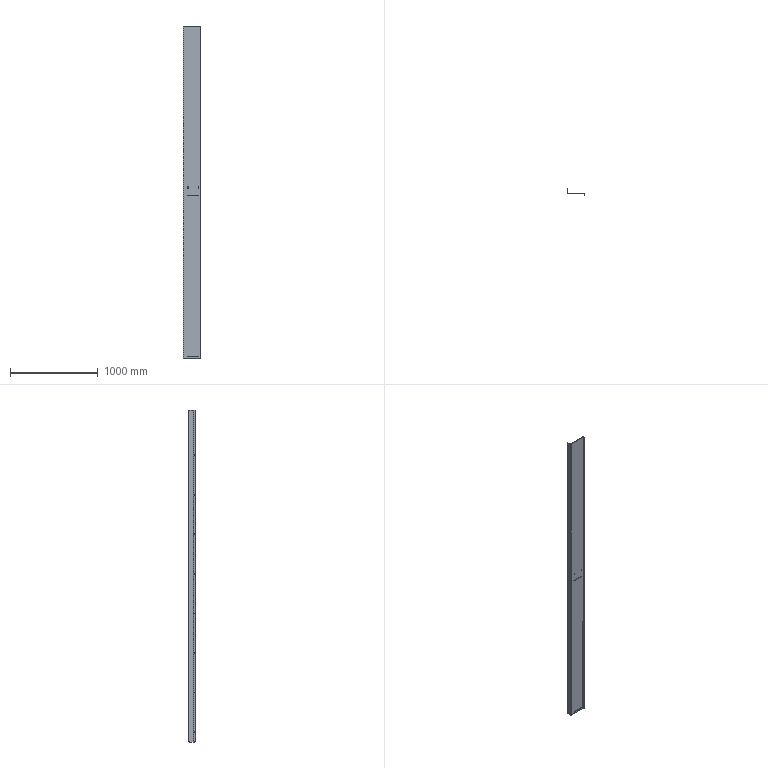Part | SolidWorks | features HoleWzd 3, Fillet 1, FlatPattern 1, ICE 1, SMBaseFlange 1, SheetMetal 1 | 1 solid | 96 faces | box 202 x 70 x 3780 mm | volume 2020331 mm3 | cylinder 82 | plane 14 | commonest cylinder face diameters 4.2 x60 6.6 x16 4 x2 8 x2 10 x2